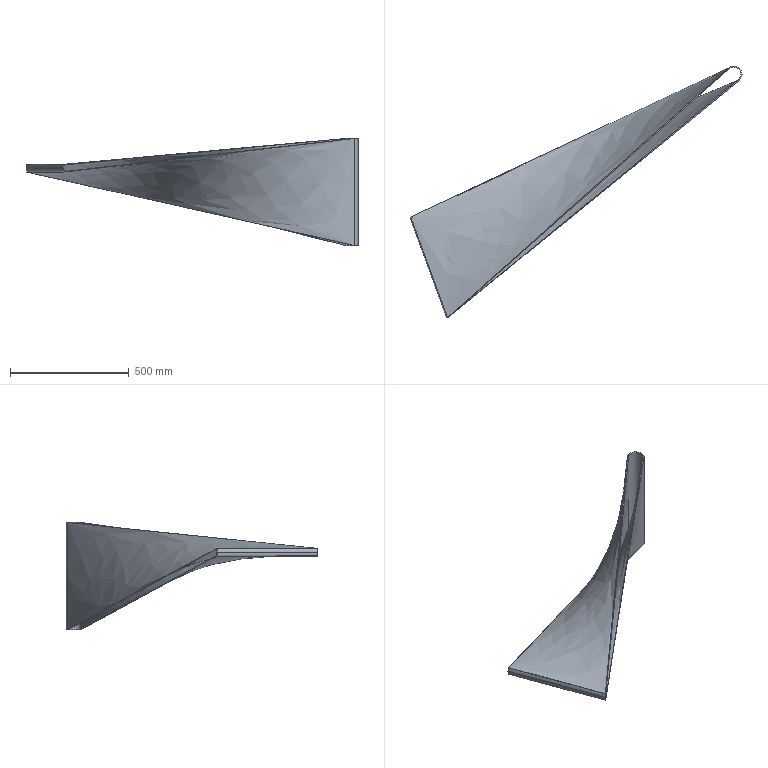Part | SolidWorks | features Blend 2, 3DProfileFeature 1, BossThin 1, ExtruThin 1 | 1 solid | 18 faces | box 1396 x 1059 x 450 mm | volume 3582512 mm3 | spline 8 | cylinder 6 | plane 4 | commonest cylinder face diameters 60 x3 70 x3
STEP:
#1=CARTESIAN_POINT('',(-1233.313,146.745,113.924));
#2=VERTEX_POINT('',#1);
#3=CARTESIAN_POINT('',(-1236.533,145.573,100.));
#4=VERTEX_POINT('',#3);
#5=CARTESIAN_POINT('',(-1208.342,155.833,100.));
#6=DIRECTION('',(0.342,-0.9397,0.));
#7=DIRECTION('',(0.9397,0.342,0.));
#8=AXIS2_PLACEMENT_3D('',#5,#6,#7);
#9=CIRCLE('',#8,30.);
#10=EDGE_CURVE('',#2,#4,#9,.T.);
#11=ORIENTED_EDGE('',*,*,#10,.T.);
#12=CARTESIAN_POINT('',(-1390.442,568.434,100.));
#13=VERTEX_POINT('',#12);
#14=CARTESIAN_POINT('',(-1236.533,145.573,100.));
#15=DIRECTION('',(-0.342,0.9397,0.));
#16=VECTOR('',#15,1000.);
#17=LINE('',#14,#16);
#18=EDGE_CURVE('',#4,#13,#17,.T.);
#19=ORIENTED_EDGE('',*,*,#18,.T.);
#20=CARTESIAN_POINT('',(-1387.222,569.606,113.924));
#21=VERTEX_POINT('',#20);
#22=CARTESIAN_POINT('',(-1362.251,578.695,100.));
#23=DIRECTION('',(0.342,-0.9397,0.));
#24=DIRECTION('',(0.9397,0.342,0.));
#25=AXIS2_PLACEMENT_3D('',#22,#23,#24);
#26=CIRCLE('',#25,30.);
#27=EDGE_CURVE('',#21,#13,#26,.T.);
#28=ORIENTED_EDGE('',*,*,#27,.F.);
#29=CARTESIAN_POINT('',(-1233.313,146.745,113.924));
#30=DIRECTION('',(-0.342,0.9397,0.));
#31=VECTOR('',#30,1000.);
#32=LINE('',#29,#31);
#33=EDGE_CURVE('',#2,#21,#32,.T.);
#34=ORIENTED_EDGE('',*,*,#33,.F.);
#35=EDGE_LOOP('',(#11,#19,#28,#34));
#36=FACE_OUTER_BOUND('',#35,.T.);
#37=CARTESIAN_POINT('',(-1208.342,155.833,100.));
#38=DIRECTION('',(-0.342,0.9397,0.));
#39=DIRECTION('',(-0.9397,-0.342,0.));
#40=AXIS2_PLACEMENT_3D('',#37,#38,#39);
#41=CYLINDRICAL_SURFACE('',#40,30.);
#42=ADVANCED_FACE('',(#36),#41,.F.);
#43=CARTESIAN_POINT('',(-1241.231,143.862,100.));
#44=VERTEX_POINT('',#43);
#45=CARTESIAN_POINT('',(-1237.474,145.23,83.756));
#46=VERTEX_POINT('',#45);
#47=CARTESIAN_POINT('',(-1208.342,155.833,100.));
#48=DIRECTION('',(0.342,-0.9397,0.));
#49=DIRECTION('',(-0.9397,-0.342,0.));
#50=AXIS2_PLACEMENT_3D('',#47,#48,#49);
#51=CIRCLE('',#50,35.);
#52=EDGE_CURVE('',#44,#46,#51,.T.);
#53=ORIENTED_EDGE('',*,*,#52,.F.);
#54=CARTESIAN_POINT('',(-1395.14,566.724,100.));
#55=VERTEX_POINT('',#54);
#56=CARTESIAN_POINT('',(-1241.231,143.862,100.));
#57=DIRECTION('',(-0.342,0.9397,0.));
#58=VECTOR('',#57,1000.);
#59=LINE('',#56,#58);
#60=EDGE_CURVE('',#44,#55,#59,.T.);
#61=ORIENTED_EDGE('',*,*,#60,.T.);
#62=CARTESIAN_POINT('',(-1391.383,568.092,83.756));
#63=VERTEX_POINT('',#62);
#64=CARTESIAN_POINT('',(-1362.251,578.695,100.));
#65=DIRECTION('',(0.342,-0.9397,0.));
#66=DIRECTION('',(-0.9397,-0.342,0.));
#67=AXIS2_PLACEMENT_3D('',#64,#65,#66);
#68=CIRCLE('',#67,35.);
#69=EDGE_CURVE('',#55,#63,#68,.T.);
#70=ORIENTED_EDGE('',*,*,#69,.T.);
#71=CARTESIAN_POINT('',(-1237.474,145.23,83.756));
#72=CARTESIAN_POINT('',(-1263.126,215.707,83.756));
#73=CARTESIAN_POINT('',(-1288.777,286.184,83.756));
#74=CARTESIAN_POINT('',(-1340.08,427.138,83.756));
#75=CARTESIAN_POINT('',(-1365.732,497.615,83.756));
#76=CARTESIAN_POINT('',(-1391.383,568.092,83.756));
#77=B_SPLINE_CURVE_WITH_KNOTS('',3,(#71,#72,#73,#74,#75,#76),.UNSPECIFIED.,.F.,.F.,(4,2,4),(0.,0.5,1.),.UNSPECIFIED.);
#78=EDGE_CURVE('',#46,#63,#77,.T.);
#79=ORIENTED_EDGE('',*,*,#78,.F.);
#80=EDGE_LOOP('',(#53,#61,#70,#79));
#81=FACE_OUTER_BOUND('',#80,.T.);
#82=CARTESIAN_POINT('',(-1208.342,155.833,100.));
#83=DIRECTION('',(-0.342,0.9397,0.));
#84=DIRECTION('',(-0.9397,-0.342,0.));
#85=AXIS2_PLACEMENT_3D('',#82,#83,#84);
#86=CYLINDRICAL_SURFACE('',#85,35.);
#87=ADVANCED_FACE('',(#81),#86,.T.);
#88=CARTESIAN_POINT('',(-14.752,1138.867,-225.));
#89=VERTEX_POINT('',#88);
#90=CARTESIAN_POINT('',(-53.546,1197.133,-225.));
#91=VERTEX_POINT('',#90);
#92=CARTESIAN_POINT('',(-34.149,1168.,-225.));
#93=DIRECTION('',(0.,0.,1.));
#94=DIRECTION('',(1.,0.,0.));
#95=AXIS2_PLACEMENT_3D('',#92,#93,#94);
#96=CIRCLE('',#95,35.);
#97=EDGE_CURVE('',#89,#91,#96,.T.);
#98=ORIENTED_EDGE('',*,*,#97,.T.);
#99=CARTESIAN_POINT('',(-53.546,1197.133,-0.8297));
#100=VERTEX_POINT('',#99);
#101=CARTESIAN_POINT('',(-53.546,1197.133,225.));
#102=DIRECTION('',(0.,0.,-1.));
#103=VECTOR('',#102,1000.);
#104=LINE('',#101,#103);
#105=EDGE_CURVE('',#100,#91,#104,.T.);
#106=ORIENTED_EDGE('',*,*,#105,.F.);
#107=CARTESIAN_POINT('',(-53.546,1197.133,225.));
#108=VERTEX_POINT('',#107);
#109=CARTESIAN_POINT('',(-53.546,1197.133,225.));
#110=DIRECTION('',(0.,0.,-1.));
#111=VECTOR('',#110,1000.);
#112=LINE('',#109,#111);
#113=EDGE_CURVE('',#108,#100,#112,.T.);
#114=ORIENTED_EDGE('',*,*,#113,.F.);
#115=CARTESIAN_POINT('',(-14.752,1138.867,225.));
#116=VERTEX_POINT('',#115);
#117=CARTESIAN_POINT('',(-34.149,1168.,225.));
#118=DIRECTION('',(0.,0.,1.));
#119=DIRECTION('',(1.,0.,0.));
#120=AXIS2_PLACEMENT_3D('',#117,#118,#119);
#121=CIRCLE('',#120,35.);
#122=EDGE_CURVE('',#116,#108,#121,.T.);
#123=ORIENTED_EDGE('',*,*,#122,.F.);
#124=CARTESIAN_POINT('',(-14.752,1138.867,225.));
#125=DIRECTION('',(0.,0.,-1.));
#126=VECTOR('',#125,1000.);
#127=LINE('',#124,#126);
#128=EDGE_CURVE('',#116,#89,#127,.T.);
#129=ORIENTED_EDGE('',*,*,#128,.T.);
#130=EDGE_LOOP('',(#98,#106,#114,#123,#129));
#131=FACE_OUTER_BOUND('',#130,.T.);
#132=CARTESIAN_POINT('',(-34.149,1168.,225.));
#133=DIRECTION('',(0.,0.,-1.));
#134=DIRECTION('',(-1.,0.,0.));
#135=AXIS2_PLACEMENT_3D('',#132,#133,#134);
#136=CYLINDRICAL_SURFACE('',#135,35.);
#137=ADVANCED_FACE('',(#131),#136,.T.);
#138=CARTESIAN_POINT('',(-17.523,1143.029,-225.));
#139=VERTEX_POINT('',#138);
#140=CARTESIAN_POINT('',(-50.775,1192.971,-225.));
#141=VERTEX_POINT('',#140);
#142=CARTESIAN_POINT('',(-34.149,1168.,-225.));
#143=DIRECTION('',(0.,0.,1.));
#144=DIRECTION('',(1.,0.,0.));
#145=AXIS2_PLACEMENT_3D('',#142,#143,#144);
#146=CIRCLE('',#145,30.);
#147=EDGE_CURVE('',#139,#141,#146,.T.);
#148=ORIENTED_EDGE('',*,*,#147,.F.);
#149=CARTESIAN_POINT('',(-17.523,1143.029,225.));
#150=VERTEX_POINT('',#149);
#151=CARTESIAN_POINT('',(-17.523,1143.029,225.));
#152=DIRECTION('',(0.,0.,-1.));
#153=VECTOR('',#152,1000.);
#154=LINE('',#151,#153);
#155=EDGE_CURVE('',#150,#139,#154,.T.);
#156=ORIENTED_EDGE('',*,*,#155,.F.);
#157=CARTESIAN_POINT('',(-50.775,1192.971,225.));
#158=VERTEX_POINT('',#157);
#159=CARTESIAN_POINT('',(-34.149,1168.,225.));
#160=DIRECTION('',(0.,0.,1.));
#161=DIRECTION('',(1.,0.,0.));
#162=AXIS2_PLACEMENT_3D('',#159,#160,#161);
#163=CIRCLE('',#162,30.);
#164=EDGE_CURVE('',#150,#158,#163,.T.);
#165=ORIENTED_EDGE('',*,*,#164,.T.);
#166=CARTESIAN_POINT('',(-50.775,1192.971,3.24));
#167=VERTEX_POINT('',#166);
#168=CARTESIAN_POINT('',(-50.775,1192.971,225.));
#169=DIRECTION('',(0.,0.,-1.));
#170=VECTOR('',#169,1000.);
#171=LINE('',#168,#170);
#172=EDGE_CURVE('',#158,#167,#171,.T.);
#173=ORIENTED_EDGE('',*,*,#172,.T.);
#174=CARTESIAN_POINT('',(-50.775,1192.971,225.));
#175=DIRECTION('',(0.,0.,-1.));
#176=VECTOR('',#175,1000.);
#177=LINE('',#174,#176);
#178=EDGE_CURVE('',#167,#141,#177,.T.);
#179=ORIENTED_EDGE('',*,*,#178,.T.);
#180=EDGE_LOOP('',(#148,#156,#165,#173,#179));
#181=FACE_OUTER_BOUND('',#180,.T.);
#182=CARTESIAN_POINT('',(-34.149,1168.,225.));
#183=DIRECTION('',(0.,0.,-1.));
#184=DIRECTION('',(-1.,0.,0.));
#185=AXIS2_PLACEMENT_3D('',#182,#183,#184);
#186=CYLINDRICAL_SURFACE('',#185,30.);
#187=ADVANCED_FACE('',(#181),#186,.F.);
#188=ORIENTED_EDGE('',*,*,#122,.T.);
#189=CARTESIAN_POINT('',(-53.546,1197.133,225.));
#190=DIRECTION('',(-0.5542,0.8324,0.));
#191=VECTOR('',#190,1000.);
#192=LINE('',#189,#191);
#193=EDGE_CURVE('',#158,#108,#192,.T.);
#194=ORIENTED_EDGE('',*,*,#193,.F.);
#195=ORIENTED_EDGE('',*,*,#164,.F.);
#196=CARTESIAN_POINT('',(-17.523,1143.029,225.));
#197=DIRECTION('',(-0.5542,0.8324,0.));
#198=VECTOR('',#197,1000.);
#199=LINE('',#196,#198);
#200=EDGE_CURVE('',#116,#150,#199,.T.);
#201=ORIENTED_EDGE('',*,*,#200,.F.);
#202=EDGE_LOOP('',(#188,#194,#195,#201));
#203=FACE_OUTER_BOUND('',#202,.T.);
#204=CARTESIAN_POINT('',(-34.149,1168.,225.));
#205=DIRECTION('',(0.,0.,1.));
#206=DIRECTION('',(1.,0.,0.));
#207=AXIS2_PLACEMENT_3D('',#204,#205,#206);
#208=PLANE('',#207);
#209=ADVANCED_FACE('',(#203),#208,.T.);
#210=ORIENTED_EDGE('',*,*,#97,.F.);
#211=CARTESIAN_POINT('',(-14.752,1138.867,-225.));
#212=DIRECTION('',(-0.5542,0.8324,0.));
#213=VECTOR('',#212,1000.);
#214=LINE('',#211,#213);
#215=EDGE_CURVE('',#89,#139,#214,.T.);
#216=ORIENTED_EDGE('',*,*,#215,.T.);
#217=ORIENTED_EDGE('',*,*,#147,.T.);
#218=CARTESIAN_POINT('',(-50.775,1192.971,-225.));
#219=DIRECTION('',(-0.5542,0.8324,0.));
#220=VECTOR('',#219,1000.);
#221=LINE('',#218,#220);
#222=EDGE_CURVE('',#141,#91,#221,.T.);
#223=ORIENTED_EDGE('',*,*,#222,.T.);
#224=EDGE_LOOP('',(#210,#216,#217,#223));
#225=FACE_OUTER_BOUND('',#224,.T.);
#226=CARTESIAN_POINT('',(-34.149,1168.,-225.));
#227=DIRECTION('',(0.,0.,1.));
#228=DIRECTION('',(1.,0.,0.));
#229=AXIS2_PLACEMENT_3D('',#226,#227,#228);
#230=PLANE('',#229);
#231=ADVANCED_FACE('',(#225),#230,.F.);
#232=ORIENTED_EDGE('',*,*,#222,.F.);
#233=CARTESIAN_POINT('',(-718.998,881.289,-55.538));
#234=DIRECTION('',(-0.8832,-0.412,0.224));
#235=VECTOR('',#234,1000.);
#236=LINE('',#233,#235);
#237=EDGE_CURVE('',#141,#21,#236,.T.);
#238=ORIENTED_EDGE('',*,*,#237,.T.);
#239=CARTESIAN_POINT('',(-1391.383,568.092,116.244));
#240=VERTEX_POINT('',#239);
#241=CARTESIAN_POINT('',(-1391.383,568.092,116.244));
#242=DIRECTION('',(0.8324,0.303,-0.4641));
#243=VECTOR('',#242,1000.);
#244=LINE('',#241,#243);
#245=EDGE_CURVE('',#240,#21,#244,.T.);
#246=ORIENTED_EDGE('',*,*,#245,.F.);
#247=CARTESIAN_POINT('',(-722.465,882.612,-54.378));
#248=DIRECTION('',(0.8818,0.4146,-0.2249));
#249=VECTOR('',#248,1000.);
#250=LINE('',#247,#249);
#251=EDGE_CURVE('',#240,#91,#250,.T.);
#252=ORIENTED_EDGE('',*,*,#251,.T.);
#253=EDGE_LOOP('',(#232,#238,#246,#252));
#254=FACE_OUTER_BOUND('',#253,.T.);
#255=CARTESIAN_POINT('',(-53.546,1197.133,-225.));
#256=CARTESIAN_POINT('',(-1391.383,568.092,116.244));
#257=CARTESIAN_POINT('',(-53.084,1196.44,-225.));
#258=CARTESIAN_POINT('',(-1390.69,568.344,115.857));
#259=CARTESIAN_POINT('',(-52.623,1195.746,-225.));
#260=CARTESIAN_POINT('',(-1389.996,568.596,115.471));
#261=CARTESIAN_POINT('',(-51.699,1194.359,-225.));
#262=CARTESIAN_POINT('',(-1388.609,569.101,114.697));
#263=CARTESIAN_POINT('',(-51.237,1193.665,-225.));
#264=CARTESIAN_POINT('',(-1387.915,569.354,114.31));
#265=CARTESIAN_POINT('',(-50.775,1192.971,-225.));
#266=CARTESIAN_POINT('',(-1387.222,569.606,113.924));
#267=B_SPLINE_SURFACE_WITH_KNOTS('',3,1,((#255,#256),(#257,#258),(#259,#260),(#261,#262),(#263,#264),(#265,#266)),.UNSPECIFIED.,.F.,.F.,.F.,(4,2,4),(2,2),(0.,0.5,1.),(0.,1.),.UNSPECIFIED.);
#268=ADVANCED_FACE('',(#254),#267,.T.);
#269=ORIENTED_EDGE('',*,*,#172,.F.);
#270=CARTESIAN_POINT('',(-642.044,669.858,169.462));
#271=DIRECTION('',(-0.7471,-0.661,-0.07018));
#272=VECTOR('',#271,1000.);
#273=LINE('',#270,#272);
#274=EDGE_CURVE('',#158,#2,#273,.T.);
#275=ORIENTED_EDGE('',*,*,#274,.T.);
#276=ORIENTED_EDGE('',*,*,#33,.T.);
#277=ORIENTED_EDGE('',*,*,#237,.F.);
#278=ORIENTED_EDGE('',*,*,#178,.F.);
#279=EDGE_LOOP('',(#269,#275,#276,#277,#278));
#280=FACE_OUTER_BOUND('',#279,.T.);
#281=CARTESIAN_POINT('',(-50.775,1192.971,-225.));
#282=CARTESIAN_POINT('',(-1387.222,569.606,113.924));
#283=CARTESIAN_POINT('',(-50.775,1192.971,-150.));
#284=CARTESIAN_POINT('',(-1361.57,499.129,113.924));
#285=CARTESIAN_POINT('',(-50.775,1192.971,-75.));
#286=CARTESIAN_POINT('',(-1335.919,428.652,113.924));
#287=CARTESIAN_POINT('',(-50.775,1192.971,75.));
#288=CARTESIAN_POINT('',(-1284.616,287.699,113.924));
#289=CARTESIAN_POINT('',(-50.775,1192.971,150.));
#290=CARTESIAN_POINT('',(-1258.964,217.222,113.924));
#291=CARTESIAN_POINT('',(-50.775,1192.971,225.));
#292=CARTESIAN_POINT('',(-1233.313,146.745,113.924));
#293=B_SPLINE_SURFACE_WITH_KNOTS('',3,1,((#281,#282),(#283,#284),(#285,#286),(#287,#288),(#289,#290),(#291,#292)),.UNSPECIFIED.,.F.,.F.,.F.,(4,2,4),(2,2),(0.,0.5,1.),(0.,1.),.UNSPECIFIED.);
#294=ADVANCED_FACE('',(#280),#293,.T.);
#295=ORIENTED_EDGE('',*,*,#113,.T.);
#296=ORIENTED_EDGE('',*,*,#105,.T.);
#297=ORIENTED_EDGE('',*,*,#251,.F.);
#298=CARTESIAN_POINT('',(-1237.474,145.23,116.244));
#299=VERTEX_POINT('',#298);
#300=CARTESIAN_POINT('',(-1237.474,145.23,116.244));
#301=DIRECTION('',(-0.342,0.9397,0.));
#302=VECTOR('',#301,1000.);
#303=LINE('',#300,#302);
#304=EDGE_CURVE('',#299,#240,#303,.T.);
#305=ORIENTED_EDGE('',*,*,#304,.F.);
#306=CARTESIAN_POINT('',(-645.51,671.182,170.622));
#307=DIRECTION('',(-0.7458,-0.6626,-0.06851));
#308=VECTOR('',#307,1000.);
#309=LINE('',#306,#308);
#310=EDGE_CURVE('',#108,#299,#309,.T.);
#311=ORIENTED_EDGE('',*,*,#310,.F.);
#312=EDGE_LOOP('',(#295,#296,#297,#305,#311));
#313=FACE_OUTER_BOUND('',#312,.T.);
#314=CARTESIAN_POINT('',(-53.546,1197.133,225.));
#315=CARTESIAN_POINT('',(-1237.474,145.23,116.244));
#316=CARTESIAN_POINT('',(-53.546,1197.133,150.));
#317=CARTESIAN_POINT('',(-1263.126,215.707,116.244));
#318=CARTESIAN_POINT('',(-53.546,1197.133,75.));
#319=CARTESIAN_POINT('',(-1288.777,286.184,116.244));
#320=CARTESIAN_POINT('',(-53.546,1197.133,-75.));
#321=CARTESIAN_POINT('',(-1340.08,427.138,116.244));
#322=CARTESIAN_POINT('',(-53.546,1197.133,-150.));
#323=CARTESIAN_POINT('',(-1365.732,497.615,116.244));
#324=CARTESIAN_POINT('',(-53.546,1197.133,-225.));
#325=CARTESIAN_POINT('',(-1391.383,568.092,116.244));
#326=B_SPLINE_SURFACE_WITH_KNOTS('',3,1,((#314,#315),(#316,#317),(#318,#319),(#320,#321),(#322,#323),(#324,#325)),.UNSPECIFIED.,.F.,.F.,.F.,(4,2,4),(2,2),(0.,0.5,1.),(0.,1.),.UNSPECIFIED.);
#327=ADVANCED_FACE('',(#313),#326,.T.);
#328=ORIENTED_EDGE('',*,*,#193,.T.);
#329=ORIENTED_EDGE('',*,*,#310,.T.);
#330=CARTESIAN_POINT('',(-1237.474,145.23,116.244));
#331=DIRECTION('',(0.8324,0.303,-0.4641));
#332=VECTOR('',#331,1000.);
#333=LINE('',#330,#332);
#334=EDGE_CURVE('',#299,#2,#333,.T.);
#335=ORIENTED_EDGE('',*,*,#334,.T.);
#336=ORIENTED_EDGE('',*,*,#274,.F.);
#337=EDGE_LOOP('',(#328,#329,#335,#336));
#338=FACE_OUTER_BOUND('',#337,.T.);
#339=CARTESIAN_POINT('',(-50.775,1192.971,225.));
#340=CARTESIAN_POINT('',(-1233.313,146.745,113.924));
#341=CARTESIAN_POINT('',(-51.237,1193.665,225.));
#342=CARTESIAN_POINT('',(-1234.006,146.492,114.31));
#343=CARTESIAN_POINT('',(-51.699,1194.359,225.));
#344=CARTESIAN_POINT('',(-1234.7,146.24,114.697));
#345=CARTESIAN_POINT('',(-52.623,1195.746,225.));
#346=CARTESIAN_POINT('',(-1236.087,145.735,115.471));
#347=CARTESIAN_POINT('',(-53.084,1196.44,225.));
#348=CARTESIAN_POINT('',(-1236.781,145.482,115.857));
#349=CARTESIAN_POINT('',(-53.546,1197.133,225.));
#350=CARTESIAN_POINT('',(-1237.474,145.23,116.244));
#351=B_SPLINE_SURFACE_WITH_KNOTS('',3,1,((#339,#340),(#341,#342),(#343,#344),(#345,#346),(#347,#348),(#349,#350)),.UNSPECIFIED.,.F.,.F.,.F.,(4,2,4),(2,2),(0.,0.5,1.),(0.,1.),.UNSPECIFIED.);
#352=ADVANCED_FACE('',(#338),#351,.T.);
#353=ORIENTED_EDGE('',*,*,#60,.F.);
#354=CARTESIAN_POINT('',(-1208.342,155.833,100.));
#355=DIRECTION('',(0.342,-0.9397,0.));
#356=DIRECTION('',(-0.9397,-0.342,0.));
#357=AXIS2_PLACEMENT_3D('',#354,#355,#356);
#358=CIRCLE('',#357,35.);
#359=EDGE_CURVE('',#299,#44,#358,.T.);
#360=ORIENTED_EDGE('',*,*,#359,.F.);
#361=ORIENTED_EDGE('',*,*,#304,.T.);
#362=CARTESIAN_POINT('',(-1362.251,578.695,100.));
#363=DIRECTION('',(0.342,-0.9397,0.));
#364=DIRECTION('',(-0.9397,-0.342,0.));
#365=AXIS2_PLACEMENT_3D('',#362,#363,#364);
#366=CIRCLE('',#365,35.);
#367=EDGE_CURVE('',#240,#55,#366,.T.);
#368=ORIENTED_EDGE('',*,*,#367,.T.);
#369=EDGE_LOOP('',(#353,#360,#361,#368));
#370=FACE_OUTER_BOUND('',#369,.T.);
#371=CARTESIAN_POINT('',(-1208.342,155.833,100.));
#372=DIRECTION('',(-0.342,0.9397,0.));
#373=DIRECTION('',(-0.9397,-0.342,0.));
#374=AXIS2_PLACEMENT_3D('',#371,#372,#373);
#375=CYLINDRICAL_SURFACE('',#374,35.);
#376=ADVANCED_FACE('',(#370),#375,.T.);
#377=ORIENTED_EDGE('',*,*,#18,.F.);
#378=CARTESIAN_POINT('',(-1233.313,146.745,86.076));
#379=VERTEX_POINT('',#378);
#380=CARTESIAN_POINT('',(-1208.342,155.833,100.));
#381=DIRECTION('',(0.342,-0.9397,0.));
#382=DIRECTION('',(0.9397,0.342,0.));
#383=AXIS2_PLACEMENT_3D('',#380,#381,#382);
#384=CIRCLE('',#383,30.);
#385=EDGE_CURVE('',#4,#379,#384,.T.);
#386=ORIENTED_EDGE('',*,*,#385,.T.);
#387=CARTESIAN_POINT('',(-1387.222,569.606,86.076));
#388=VERTEX_POINT('',#387);
#389=CARTESIAN_POINT('',(-1233.313,146.745,86.076));
#390=CARTESIAN_POINT('',(-1284.616,287.699,86.076));
#391=CARTESIAN_POINT('',(-1335.919,428.652,86.076));
#392=CARTESIAN_POINT('',(-1387.222,569.606,86.076));
#393=B_SPLINE_CURVE_WITH_KNOTS('',3,(#389,#390,#391,#392),.UNSPECIFIED.,.F.,.F.,(4,4),(0.,1.),.UNSPECIFIED.);
#394=EDGE_CURVE('',#379,#388,#393,.T.);
#395=ORIENTED_EDGE('',*,*,#394,.T.);
#396=CARTESIAN_POINT('',(-1362.251,578.695,100.));
#397=DIRECTION('',(0.342,-0.9397,0.));
#398=DIRECTION('',(0.9397,0.342,0.));
#399=AXIS2_PLACEMENT_3D('',#396,#397,#398);
#400=CIRCLE('',#399,30.);
#401=EDGE_CURVE('',#13,#388,#400,.T.);
#402=ORIENTED_EDGE('',*,*,#401,.F.);
#403=EDGE_LOOP('',(#377,#386,#395,#402));
#404=FACE_OUTER_BOUND('',#403,.T.);
#405=CARTESIAN_POINT('',(-1208.342,155.833,100.));
#406=DIRECTION('',(-0.342,0.9397,0.));
#407=DIRECTION('',(-0.9397,-0.342,0.));
#408=AXIS2_PLACEMENT_3D('',#405,#406,#407);
#409=CYLINDRICAL_SURFACE('',#408,30.);
#410=ADVANCED_FACE('',(#404),#409,.F.);
#411=ORIENTED_EDGE('',*,*,#359,.T.);
#412=ORIENTED_EDGE('',*,*,#52,.T.);
#413=CARTESIAN_POINT('',(-1233.313,146.745,86.076));
#414=CARTESIAN_POINT('',(-1234.006,146.492,85.69));
#415=CARTESIAN_POINT('',(-1234.7,146.24,85.303));
#416=CARTESIAN_POINT('',(-1236.087,145.735,84.529));
#417=CARTESIAN_POINT('',(-1236.781,145.482,84.143));
#418=CARTESIAN_POINT('',(-1237.474,145.23,83.756));
#419=B_SPLINE_CURVE_WITH_KNOTS('',3,(#413,#414,#415,#416,#417,#418),.UNSPECIFIED.,.F.,.F.,(4,2,4),(0.,0.5,1.),.UNSPECIFIED.);
#420=EDGE_CURVE('',#379,#46,#419,.T.);
#421=ORIENTED_EDGE('',*,*,#420,.F.);
#422=ORIENTED_EDGE('',*,*,#385,.F.);
#423=ORIENTED_EDGE('',*,*,#10,.F.);
#424=ORIENTED_EDGE('',*,*,#334,.F.);
#425=EDGE_LOOP('',(#411,#412,#421,#422,#423,#424));
#426=FACE_OUTER_BOUND('',#425,.T.);
#427=CARTESIAN_POINT('',(-1208.342,155.833,100.));
#428=DIRECTION('',(0.342,-0.9397,0.));
#429=DIRECTION('',(-0.9397,-0.342,0.));
#430=AXIS2_PLACEMENT_3D('',#427,#428,#429);
#431=PLANE('',#430);
#432=ADVANCED_FACE('',(#426),#431,.T.);
#433=ORIENTED_EDGE('',*,*,#367,.F.);
#434=ORIENTED_EDGE('',*,*,#245,.T.);
#435=ORIENTED_EDGE('',*,*,#27,.T.);
#436=ORIENTED_EDGE('',*,*,#401,.T.);
#437=CARTESIAN_POINT('',(-1387.222,569.606,86.076));
#438=CARTESIAN_POINT('',(-1388.609,569.101,85.303));
#439=CARTESIAN_POINT('',(-1389.996,568.596,84.529));
#440=CARTESIAN_POINT('',(-1391.383,568.092,83.756));
#441=B_SPLINE_CURVE_WITH_KNOTS('',3,(#437,#438,#439,#440),.UNSPECIFIED.,.F.,.F.,(4,4),(0.,1.),.UNSPECIFIED.);
#442=EDGE_CURVE('',#388,#63,#441,.T.);
#443=ORIENTED_EDGE('',*,*,#442,.T.);
#444=ORIENTED_EDGE('',*,*,#69,.F.);
#445=EDGE_LOOP('',(#433,#434,#435,#436,#443,#444));
#446=FACE_OUTER_BOUND('',#445,.T.);
#447=CARTESIAN_POINT('',(-1362.251,578.695,100.));
#448=DIRECTION('',(0.342,-0.9397,0.));
#449=DIRECTION('',(-0.9397,-0.342,0.));
#450=AXIS2_PLACEMENT_3D('',#447,#448,#449);
#451=PLANE('',#450);
#452=ADVANCED_FACE('',(#446),#451,.F.);
#453=ORIENTED_EDGE('',*,*,#128,.F.);
#454=CARTESIAN_POINT('',(-626.113,642.048,154.378));
#455=DIRECTION('',(-0.773,-0.6281,-0.08929));
#456=VECTOR('',#455,1000.);
#457=LINE('',#454,#456);
#458=EDGE_CURVE('',#116,#46,#457,.T.);
#459=ORIENTED_EDGE('',*,*,#458,.T.);
#460=ORIENTED_EDGE('',*,*,#78,.T.);
#461=CARTESIAN_POINT('',(-703.068,853.479,-70.622));
#462=DIRECTION('',(0.9045,0.375,-0.2029));
#463=VECTOR('',#462,1000.);
#464=LINE('',#461,#463);
#465=EDGE_CURVE('',#63,#89,#464,.T.);
#466=ORIENTED_EDGE('',*,*,#465,.T.);
#467=EDGE_LOOP('',(#453,#459,#460,#466));
#468=FACE_OUTER_BOUND('',#467,.T.);
#469=CARTESIAN_POINT('',(-14.752,1138.867,-225.));
#470=CARTESIAN_POINT('',(-1391.383,568.092,83.756));
#471=CARTESIAN_POINT('',(-14.752,1138.867,-150.));
#472=CARTESIAN_POINT('',(-1365.732,497.615,83.756));
#473=CARTESIAN_POINT('',(-14.752,1138.867,-75.));
#474=CARTESIAN_POINT('',(-1340.08,427.138,83.756));
#475=CARTESIAN_POINT('',(-14.752,1138.867,75.));
#476=CARTESIAN_POINT('',(-1288.777,286.184,83.756));
#477=CARTESIAN_POINT('',(-14.752,1138.867,150.));
#478=CARTESIAN_POINT('',(-1263.126,215.707,83.756));
#479=CARTESIAN_POINT('',(-14.752,1138.867,225.));
#480=CARTESIAN_POINT('',(-1237.474,145.23,83.756));
#481=B_SPLINE_SURFACE_WITH_KNOTS('',3,1,((#469,#470),(#471,#472),(#473,#474),(#475,#476),(#477,#478),(#479,#480)),.UNSPECIFIED.,.F.,.F.,.F.,(4,2,4),(2,2),(0.,0.5,1.),(0.,1.),.UNSPECIFIED.);
#482=ADVANCED_FACE('',(#468),#481,.T.);
#483=ORIENTED_EDGE('',*,*,#200,.T.);
#484=CARTESIAN_POINT('',(-625.418,644.887,155.538));
#485=DIRECTION('',(-0.7705,-0.6314,-0.08804));
#486=VECTOR('',#485,1000.);
#487=LINE('',#484,#486);
#488=EDGE_CURVE('',#150,#379,#487,.T.);
#489=ORIENTED_EDGE('',*,*,#488,.T.);
#490=ORIENTED_EDGE('',*,*,#420,.T.);
#491=ORIENTED_EDGE('',*,*,#458,.F.);
#492=EDGE_LOOP('',(#483,#489,#490,#491));
#493=FACE_OUTER_BOUND('',#492,.T.);
#494=CARTESIAN_POINT('',(-14.752,1138.867,225.));
#495=CARTESIAN_POINT('',(-1237.474,145.23,83.756));
#496=CARTESIAN_POINT('',(-15.214,1139.56,225.));
#497=CARTESIAN_POINT('',(-1236.781,145.482,84.143));
#498=CARTESIAN_POINT('',(-15.676,1140.254,225.));
#499=CARTESIAN_POINT('',(-1236.087,145.735,84.529));
#500=CARTESIAN_POINT('',(-16.599,1141.641,225.));
#501=CARTESIAN_POINT('',(-1234.7,146.24,85.303));
#502=CARTESIAN_POINT('',(-17.061,1142.335,225.));
#503=CARTESIAN_POINT('',(-1234.006,146.492,85.69));
#504=CARTESIAN_POINT('',(-17.523,1143.029,225.));
#505=CARTESIAN_POINT('',(-1233.313,146.745,86.076));
#506=B_SPLINE_SURFACE_WITH_KNOTS('',3,1,((#494,#495),(#496,#497),(#498,#499),(#500,#501),(#502,#503),(#504,#505)),.UNSPECIFIED.,.F.,.F.,.F.,(4,2,4),(2,2),(0.,0.5,1.),(0.,1.),.UNSPECIFIED.);
#507=ADVANCED_FACE('',(#493),#506,.T.);
#508=ORIENTED_EDGE('',*,*,#215,.F.);
#509=ORIENTED_EDGE('',*,*,#465,.F.);
#510=ORIENTED_EDGE('',*,*,#442,.F.);
#511=CARTESIAN_POINT('',(-702.372,856.317,-69.462));
#512=DIRECTION('',(-0.9028,-0.378,0.205));
#513=VECTOR('',#512,1000.);
#514=LINE('',#511,#513);
#515=EDGE_CURVE('',#139,#388,#514,.T.);
#516=ORIENTED_EDGE('',*,*,#515,.F.);
#517=EDGE_LOOP('',(#508,#509,#510,#516));
#518=FACE_OUTER_BOUND('',#517,.T.);
#519=CARTESIAN_POINT('',(-17.523,1143.029,-225.));
#520=CARTESIAN_POINT('',(-1387.222,569.606,86.076));
#521=CARTESIAN_POINT('',(-17.061,1142.335,-225.));
#522=CARTESIAN_POINT('',(-1387.915,569.354,85.69));
#523=CARTESIAN_POINT('',(-16.599,1141.641,-225.));
#524=CARTESIAN_POINT('',(-1388.609,569.101,85.303));
#525=CARTESIAN_POINT('',(-15.676,1140.254,-225.));
#526=CARTESIAN_POINT('',(-1389.996,568.596,84.529));
#527=CARTESIAN_POINT('',(-15.214,1139.56,-225.));
#528=CARTESIAN_POINT('',(-1390.69,568.344,84.143));
#529=CARTESIAN_POINT('',(-14.752,1138.867,-225.));
#530=CARTESIAN_POINT('',(-1391.383,568.092,83.756));
#531=B_SPLINE_SURFACE_WITH_KNOTS('',3,1,((#519,#520),(#521,#522),(#523,#524),(#525,#526),(#527,#528),(#529,#530)),.UNSPECIFIED.,.F.,.F.,.F.,(4,2,4),(2,2),(0.,0.5,1.),(0.,1.),.UNSPECIFIED.);
#532=ADVANCED_FACE('',(#518),#531,.T.);
#533=ORIENTED_EDGE('',*,*,#155,.T.);
#534=ORIENTED_EDGE('',*,*,#515,.T.);
#535=ORIENTED_EDGE('',*,*,#394,.F.);
#536=ORIENTED_EDGE('',*,*,#488,.F.);
#537=EDGE_LOOP('',(#533,#534,#535,#536));
#538=FACE_OUTER_BOUND('',#537,.T.);
#539=CARTESIAN_POINT('',(-17.523,1143.029,225.));
#540=CARTESIAN_POINT('',(-1233.313,146.745,86.076));
#541=CARTESIAN_POINT('',(-17.523,1143.029,150.));
#542=CARTESIAN_POINT('',(-1258.964,217.222,86.076));
#543=CARTESIAN_POINT('',(-17.523,1143.029,75.));
#544=CARTESIAN_POINT('',(-1284.616,287.699,86.076));
#545=CARTESIAN_POINT('',(-17.523,1143.029,-75.));
#546=CARTESIAN_POINT('',(-1335.919,428.652,86.076));
#547=CARTESIAN_POINT('',(-17.523,1143.029,-150.));
#548=CARTESIAN_POINT('',(-1361.57,499.129,86.076));
#549=CARTESIAN_POINT('',(-17.523,1143.029,-225.));
#550=CARTESIAN_POINT('',(-1387.222,569.606,86.076));
#551=B_SPLINE_SURFACE_WITH_KNOTS('',3,1,((#539,#540),(#541,#542),(#543,#544),(#545,#546),(#547,#548),(#549,#550)),.UNSPECIFIED.,.F.,.F.,.F.,(4,2,4),(2,2),(0.,0.5,1.),(0.,1.),.UNSPECIFIED.);
#552=ADVANCED_FACE('',(#538),#551,.T.);
#553=CLOSED_SHELL('',(#42,#87,#137,#187,#209,#231,#268,#294,#327,#352,#376,#410,#432,#452,#482,#507,#532,#552));
#554=MANIFOLD_SOLID_BREP('',#553);
#555=CARTESIAN_POINT('',(0.,0.,0.));
#556=DIRECTION('',(0.,0.,1.));
#557=DIRECTION('',(1.,0.,0.));
#558=AXIS2_PLACEMENT_3D('',#555,#556,#557);
#559=(LENGTH_UNIT()NAMED_UNIT(*)SI_UNIT(.MILLI.,.METRE.));
#560=UNCERTAINTY_MEASURE_WITH_UNIT(LENGTH_MEASURE(0.00001),#559,'','');
#561=(NAMED_UNIT(*)PLANE_ANGLE_UNIT()SI_UNIT($,.RADIAN.));
#562=(NAMED_UNIT(*)SI_UNIT($,.STERADIAN.)SOLID_ANGLE_UNIT());
#563=(GEOMETRIC_REPRESENTATION_CONTEXT(3)GLOBAL_UNCERTAINTY_ASSIGNED_CONTEXT((#560))GLOBAL_UNIT_ASSIGNED_CONTEXT((#559,#561,#562))REPRESENTATION_CONTEXT('',''));
#564=ADVANCED_BREP_SHAPE_REPRESENTATION('',(#554,#558),#563);